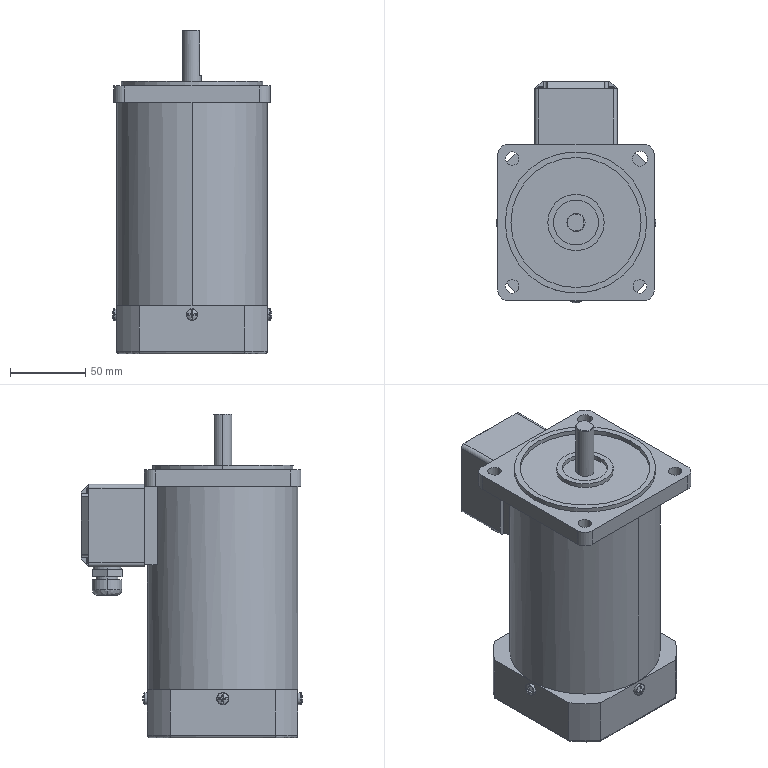Part | SolidWorks | features BaseBody 1, HoleWzd 1 | 1 solid | 258 faces | box 106.313 x 147.157 x 215 mm | volume 1631430 mm3 | plane 162 | cylinder 64 | spline 30 | cone 2 | commonest cylinder face diameters 4.125 x12 8 x8 9 x6 3.12 x4 5.5 x4 14.56 x4